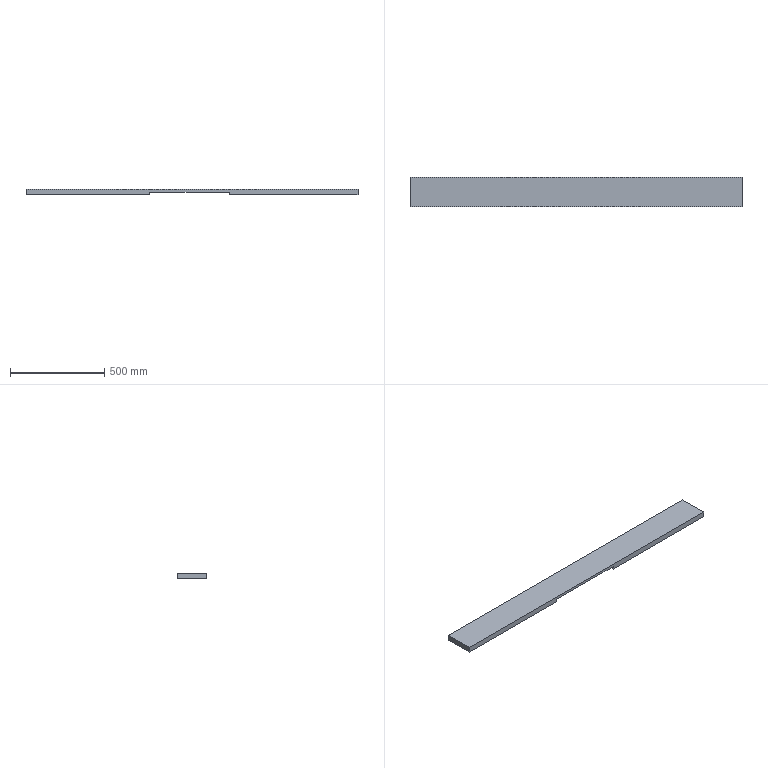Part | NX | features BREP 1 | 1 solid | 10 faces | box 1764 x 158 x 30 mm | volume 7354110 mm3 | plane 10
STEP:
#1=CARTESIAN_POINT('',(-225.5,79.,-15.));
#2=VERTEX_POINT('',#1);
#3=CARTESIAN_POINT('',(-882.,79.,-15.));
#4=VERTEX_POINT('',#3);
#5=CARTESIAN_POINT('',(-882.,79.,-15.));
#6=DIRECTION('',(-1.,0.,0.));
#7=VECTOR('',#6,1000.);
#8=LINE('',#5,#7);
#9=EDGE_CURVE('',#2,#4,#8,.T.);
#10=ORIENTED_EDGE('',*,*,#9,.F.);
#11=CARTESIAN_POINT('',(-225.5,-79.,-15.));
#12=VERTEX_POINT('',#11);
#13=CARTESIAN_POINT('',(-225.5,79.,-15.));
#14=DIRECTION('',(0.,1.,0.));
#15=VECTOR('',#14,1000.);
#16=LINE('',#13,#15);
#17=EDGE_CURVE('',#12,#2,#16,.T.);
#18=ORIENTED_EDGE('',*,*,#17,.F.);
#19=CARTESIAN_POINT('',(-882.,-79.,-15.));
#20=VERTEX_POINT('',#19);
#21=CARTESIAN_POINT('',(-882.,-79.,-15.));
#22=DIRECTION('',(1.,0.,0.));
#23=VECTOR('',#22,1000.);
#24=LINE('',#21,#23);
#25=EDGE_CURVE('',#20,#12,#24,.T.);
#26=ORIENTED_EDGE('',*,*,#25,.F.);
#27=CARTESIAN_POINT('',(-882.,79.,-15.));
#28=DIRECTION('',(0.,-1.,0.));
#29=VECTOR('',#28,1000.);
#30=LINE('',#27,#29);
#31=EDGE_CURVE('',#4,#20,#30,.T.);
#32=ORIENTED_EDGE('',*,*,#31,.F.);
#33=EDGE_LOOP('',(#10,#18,#26,#32));
#34=FACE_BOUND('',#33,.T.);
#35=CARTESIAN_POINT('',(-882.,-79.,-15.));
#36=DIRECTION('',(0.,0.,1.));
#37=DIRECTION('',(-1.,0.,0.));
#38=AXIS2_PLACEMENT_3D('',#35,#36,#37);
#39=PLANE('',#38);
#40=ADVANCED_FACE('',(#34),#39,.F.);
#41=ORIENTED_EDGE('',*,*,#31,.T.);
#42=CARTESIAN_POINT('',(-882.,-79.,15.));
#43=VERTEX_POINT('',#42);
#44=CARTESIAN_POINT('',(-882.,-79.,15.));
#45=DIRECTION('',(0.,0.,-1.));
#46=VECTOR('',#45,1000.);
#47=LINE('',#44,#46);
#48=EDGE_CURVE('',#43,#20,#47,.T.);
#49=ORIENTED_EDGE('',*,*,#48,.F.);
#50=CARTESIAN_POINT('',(-882.,79.,15.));
#51=VERTEX_POINT('',#50);
#52=CARTESIAN_POINT('',(-882.,79.,15.));
#53=DIRECTION('',(0.,-1.,0.));
#54=VECTOR('',#53,1000.);
#55=LINE('',#52,#54);
#56=EDGE_CURVE('',#51,#43,#55,.T.);
#57=ORIENTED_EDGE('',*,*,#56,.F.);
#58=CARTESIAN_POINT('',(-882.,79.,15.));
#59=DIRECTION('',(0.,0.,-1.));
#60=VECTOR('',#59,1000.);
#61=LINE('',#58,#60);
#62=EDGE_CURVE('',#51,#4,#61,.T.);
#63=ORIENTED_EDGE('',*,*,#62,.T.);
#64=EDGE_LOOP('',(#41,#49,#57,#63));
#65=FACE_BOUND('',#64,.T.);
#66=CARTESIAN_POINT('',(-882.,79.,15.));
#67=DIRECTION('',(1.,0.,0.));
#68=DIRECTION('',(0.,0.,1.));
#69=AXIS2_PLACEMENT_3D('',#66,#67,#68);
#70=PLANE('',#69);
#71=ADVANCED_FACE('',(#65),#70,.F.);
#72=ORIENTED_EDGE('',*,*,#25,.T.);
#73=CARTESIAN_POINT('',(-225.5,-79.,0.));
#74=VERTEX_POINT('',#73);
#75=CARTESIAN_POINT('',(-225.5,-79.,0.));
#76=DIRECTION('',(0.,0.,-1.));
#77=VECTOR('',#76,1000.);
#78=LINE('',#75,#77);
#79=EDGE_CURVE('',#74,#12,#78,.T.);
#80=ORIENTED_EDGE('',*,*,#79,.F.);
#81=CARTESIAN_POINT('',(199.5,-79.,0.));
#82=VERTEX_POINT('',#81);
#83=CARTESIAN_POINT('',(-225.5,-79.,0.));
#84=DIRECTION('',(-1.,0.,0.));
#85=VECTOR('',#84,1000.);
#86=LINE('',#83,#85);
#87=EDGE_CURVE('',#82,#74,#86,.T.);
#88=ORIENTED_EDGE('',*,*,#87,.F.);
#89=CARTESIAN_POINT('',(199.5,-79.,-15.));
#90=VERTEX_POINT('',#89);
#91=CARTESIAN_POINT('',(199.5,-79.,0.));
#92=DIRECTION('',(0.,0.,-1.));
#93=VECTOR('',#92,1000.);
#94=LINE('',#91,#93);
#95=EDGE_CURVE('',#82,#90,#94,.T.);
#96=ORIENTED_EDGE('',*,*,#95,.T.);
#97=CARTESIAN_POINT('',(882.,-79.,-15.));
#98=VERTEX_POINT('',#97);
#99=CARTESIAN_POINT('',(-882.,-79.,-15.));
#100=DIRECTION('',(1.,0.,0.));
#101=VECTOR('',#100,1000.);
#102=LINE('',#99,#101);
#103=EDGE_CURVE('',#90,#98,#102,.T.);
#104=ORIENTED_EDGE('',*,*,#103,.T.);
#105=CARTESIAN_POINT('',(882.,-79.,15.));
#106=VERTEX_POINT('',#105);
#107=CARTESIAN_POINT('',(882.,-79.,15.));
#108=DIRECTION('',(0.,0.,-1.));
#109=VECTOR('',#108,1000.);
#110=LINE('',#107,#109);
#111=EDGE_CURVE('',#106,#98,#110,.T.);
#112=ORIENTED_EDGE('',*,*,#111,.F.);
#113=CARTESIAN_POINT('',(-882.,-79.,15.));
#114=DIRECTION('',(1.,0.,0.));
#115=VECTOR('',#114,1000.);
#116=LINE('',#113,#115);
#117=EDGE_CURVE('',#43,#106,#116,.T.);
#118=ORIENTED_EDGE('',*,*,#117,.F.);
#119=ORIENTED_EDGE('',*,*,#48,.T.);
#120=EDGE_LOOP('',(#72,#80,#88,#96,#104,#112,#118,#119));
#121=FACE_BOUND('',#120,.T.);
#122=CARTESIAN_POINT('',(-882.,-79.,15.));
#123=DIRECTION('',(0.,1.,0.));
#124=DIRECTION('',(0.,0.,-1.));
#125=AXIS2_PLACEMENT_3D('',#122,#123,#124);
#126=PLANE('',#125);
#127=ADVANCED_FACE('',(#121),#126,.F.);
#128=CARTESIAN_POINT('',(882.,79.,-15.));
#129=VERTEX_POINT('',#128);
#130=CARTESIAN_POINT('',(882.,79.,-15.));
#131=DIRECTION('',(0.,1.,0.));
#132=VECTOR('',#131,1000.);
#133=LINE('',#130,#132);
#134=EDGE_CURVE('',#98,#129,#133,.T.);
#135=ORIENTED_EDGE('',*,*,#134,.T.);
#136=CARTESIAN_POINT('',(882.,79.,15.));
#137=VERTEX_POINT('',#136);
#138=CARTESIAN_POINT('',(882.,79.,15.));
#139=DIRECTION('',(0.,0.,-1.));
#140=VECTOR('',#139,1000.);
#141=LINE('',#138,#140);
#142=EDGE_CURVE('',#137,#129,#141,.T.);
#143=ORIENTED_EDGE('',*,*,#142,.F.);
#144=CARTESIAN_POINT('',(882.,79.,15.));
#145=DIRECTION('',(0.,1.,0.));
#146=VECTOR('',#145,1000.);
#147=LINE('',#144,#146);
#148=EDGE_CURVE('',#106,#137,#147,.T.);
#149=ORIENTED_EDGE('',*,*,#148,.F.);
#150=ORIENTED_EDGE('',*,*,#111,.T.);
#151=EDGE_LOOP('',(#135,#143,#149,#150));
#152=FACE_BOUND('',#151,.T.);
#153=CARTESIAN_POINT('',(882.,79.,15.));
#154=DIRECTION('',(-1.,0.,0.));
#155=DIRECTION('',(0.,0.,-1.));
#156=AXIS2_PLACEMENT_3D('',#153,#154,#155);
#157=PLANE('',#156);
#158=ADVANCED_FACE('',(#152),#157,.F.);
#159=CARTESIAN_POINT('',(-225.5,79.,0.));
#160=VERTEX_POINT('',#159);
#161=CARTESIAN_POINT('',(199.5,79.,0.));
#162=VERTEX_POINT('',#161);
#163=CARTESIAN_POINT('',(-225.5,79.,0.));
#164=DIRECTION('',(1.,0.,0.));
#165=VECTOR('',#164,1000.);
#166=LINE('',#163,#165);
#167=EDGE_CURVE('',#160,#162,#166,.T.);
#168=ORIENTED_EDGE('',*,*,#167,.F.);
#169=CARTESIAN_POINT('',(-225.5,79.,0.));
#170=DIRECTION('',(0.,0.,-1.));
#171=VECTOR('',#170,1000.);
#172=LINE('',#169,#171);
#173=EDGE_CURVE('',#160,#2,#172,.T.);
#174=ORIENTED_EDGE('',*,*,#173,.T.);
#175=ORIENTED_EDGE('',*,*,#9,.T.);
#176=ORIENTED_EDGE('',*,*,#62,.F.);
#177=CARTESIAN_POINT('',(-882.,79.,15.));
#178=DIRECTION('',(-1.,0.,0.));
#179=VECTOR('',#178,1000.);
#180=LINE('',#177,#179);
#181=EDGE_CURVE('',#137,#51,#180,.T.);
#182=ORIENTED_EDGE('',*,*,#181,.F.);
#183=ORIENTED_EDGE('',*,*,#142,.T.);
#184=CARTESIAN_POINT('',(199.5,79.,-15.));
#185=VERTEX_POINT('',#184);
#186=CARTESIAN_POINT('',(-882.,79.,-15.));
#187=DIRECTION('',(-1.,0.,0.));
#188=VECTOR('',#187,1000.);
#189=LINE('',#186,#188);
#190=EDGE_CURVE('',#129,#185,#189,.T.);
#191=ORIENTED_EDGE('',*,*,#190,.T.);
#192=CARTESIAN_POINT('',(199.5,79.,0.));
#193=DIRECTION('',(0.,0.,-1.));
#194=VECTOR('',#193,1000.);
#195=LINE('',#192,#194);
#196=EDGE_CURVE('',#162,#185,#195,.T.);
#197=ORIENTED_EDGE('',*,*,#196,.F.);
#198=EDGE_LOOP('',(#168,#174,#175,#176,#182,#183,#191,#197));
#199=FACE_BOUND('',#198,.T.);
#200=CARTESIAN_POINT('',(-882.,79.,15.));
#201=DIRECTION('',(0.,-1.,0.));
#202=DIRECTION('',(0.,0.,1.));
#203=AXIS2_PLACEMENT_3D('',#200,#201,#202);
#204=PLANE('',#203);
#205=ADVANCED_FACE('',(#199),#204,.F.);
#206=ORIENTED_EDGE('',*,*,#56,.T.);
#207=ORIENTED_EDGE('',*,*,#117,.T.);
#208=ORIENTED_EDGE('',*,*,#148,.T.);
#209=ORIENTED_EDGE('',*,*,#181,.T.);
#210=EDGE_LOOP('',(#206,#207,#208,#209));
#211=FACE_BOUND('',#210,.T.);
#212=CARTESIAN_POINT('',(-882.,-79.,15.));
#213=DIRECTION('',(0.,0.,1.));
#214=DIRECTION('',(-1.,0.,0.));
#215=AXIS2_PLACEMENT_3D('',#212,#213,#214);
#216=PLANE('',#215);
#217=ADVANCED_FACE('',(#211),#216,.T.);
#218=ORIENTED_EDGE('',*,*,#103,.F.);
#219=CARTESIAN_POINT('',(199.5,79.,-15.));
#220=DIRECTION('',(0.,-1.,0.));
#221=VECTOR('',#220,1000.);
#222=LINE('',#219,#221);
#223=EDGE_CURVE('',#185,#90,#222,.T.);
#224=ORIENTED_EDGE('',*,*,#223,.F.);
#225=ORIENTED_EDGE('',*,*,#190,.F.);
#226=ORIENTED_EDGE('',*,*,#134,.F.);
#227=EDGE_LOOP('',(#218,#224,#225,#226));
#228=FACE_BOUND('',#227,.T.);
#229=CARTESIAN_POINT('',(-882.,-79.,-15.));
#230=DIRECTION('',(0.,0.,1.));
#231=DIRECTION('',(-1.,0.,0.));
#232=AXIS2_PLACEMENT_3D('',#229,#230,#231);
#233=PLANE('',#232);
#234=ADVANCED_FACE('',(#228),#233,.F.);
#235=ORIENTED_EDGE('',*,*,#17,.T.);
#236=ORIENTED_EDGE('',*,*,#173,.F.);
#237=CARTESIAN_POINT('',(-225.5,79.,0.));
#238=DIRECTION('',(0.,1.,0.));
#239=VECTOR('',#238,1000.);
#240=LINE('',#237,#239);
#241=EDGE_CURVE('',#74,#160,#240,.T.);
#242=ORIENTED_EDGE('',*,*,#241,.F.);
#243=ORIENTED_EDGE('',*,*,#79,.T.);
#244=EDGE_LOOP('',(#235,#236,#242,#243));
#245=FACE_BOUND('',#244,.T.);
#246=CARTESIAN_POINT('',(-225.5,79.,0.));
#247=DIRECTION('',(-1.,0.,0.));
#248=DIRECTION('',(0.,1.,0.));
#249=AXIS2_PLACEMENT_3D('',#246,#247,#248);
#250=PLANE('',#249);
#251=ADVANCED_FACE('',(#245),#250,.F.);
#252=ORIENTED_EDGE('',*,*,#223,.T.);
#253=ORIENTED_EDGE('',*,*,#95,.F.);
#254=CARTESIAN_POINT('',(199.5,79.,0.));
#255=DIRECTION('',(0.,-1.,0.));
#256=VECTOR('',#255,1000.);
#257=LINE('',#254,#256);
#258=EDGE_CURVE('',#162,#82,#257,.T.);
#259=ORIENTED_EDGE('',*,*,#258,.F.);
#260=ORIENTED_EDGE('',*,*,#196,.T.);
#261=EDGE_LOOP('',(#252,#253,#259,#260));
#262=FACE_BOUND('',#261,.T.);
#263=CARTESIAN_POINT('',(199.5,79.,0.));
#264=DIRECTION('',(1.,0.,0.));
#265=DIRECTION('',(0.,-1.,0.));
#266=AXIS2_PLACEMENT_3D('',#263,#264,#265);
#267=PLANE('',#266);
#268=ADVANCED_FACE('',(#262),#267,.F.);
#269=ORIENTED_EDGE('',*,*,#241,.T.);
#270=ORIENTED_EDGE('',*,*,#167,.T.);
#271=ORIENTED_EDGE('',*,*,#258,.T.);
#272=ORIENTED_EDGE('',*,*,#87,.T.);
#273=EDGE_LOOP('',(#269,#270,#271,#272));
#274=FACE_BOUND('',#273,.T.);
#275=CARTESIAN_POINT('',(-225.5,79.,0.));
#276=DIRECTION('',(0.,0.,1.));
#277=DIRECTION('',(-1.,0.,0.));
#278=AXIS2_PLACEMENT_3D('',#275,#276,#277);
#279=PLANE('',#278);
#280=ADVANCED_FACE('',(#274),#279,.F.);
#281=CLOSED_SHELL('',(#40,#71,#127,#158,#205,#217,#234,#251,#268,#280));
#282=MANIFOLD_SOLID_BREP('',#281);
#283=(LENGTH_UNIT()NAMED_UNIT(*)SI_UNIT(.MILLI.,.METRE.));
#284=UNCERTAINTY_MEASURE_WITH_UNIT(LENGTH_MEASURE(0.00001),#283,'','');
#285=(NAMED_UNIT(*)PLANE_ANGLE_UNIT()SI_UNIT($,.RADIAN.));
#286=(NAMED_UNIT(*)SI_UNIT($,.STERADIAN.)SOLID_ANGLE_UNIT());
#287=(GEOMETRIC_REPRESENTATION_CONTEXT(3)GLOBAL_UNCERTAINTY_ASSIGNED_CONTEXT((#284))GLOBAL_UNIT_ASSIGNED_CONTEXT((#283,#285,#286))REPRESENTATION_CONTEXT('',''));
#288=ADVANCED_BREP_SHAPE_REPRESENTATION('',(#282),#287);